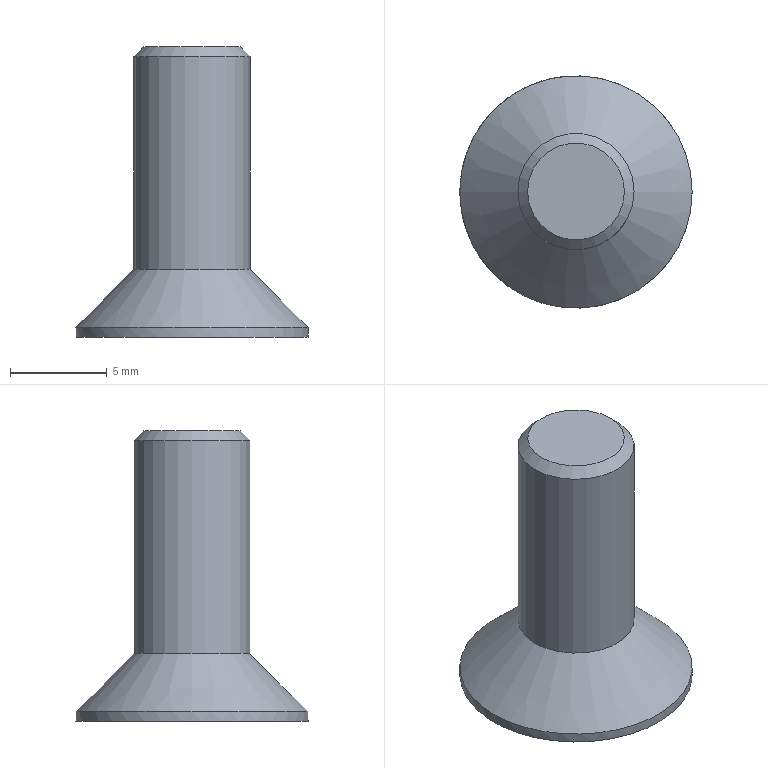Part | STEP file | LJD_id162_x_t | 1 solid | 13 faces | box 12 x 12 x 15 mm | volume 521.973 mm3 | plane 9 | cylinder 2 | cone 2 | commonest cylinder face diameters 6 x1 12 x1
STEP:
#1=CARTESIAN_POINT('',(61.,0.,-165.25));
#2=VERTEX_POINT('',#1);
#3=CARTESIAN_POINT('',(55.,0.,-165.25));
#4=DIRECTION('',(0.,0.,1.));
#5=DIRECTION('',(1.,0.,0.));
#6=AXIS2_PLACEMENT_3D('',#3,#4,#5);
#7=CIRCLE('',#6,6.);
#8=EDGE_CURVE('',#2,#2,#7,.T.);
#9=ORIENTED_EDGE('',*,*,#8,.F.);
#10=EDGE_LOOP('',(#9));
#11=FACE_BOUND('',#10,.T.);
#12=CARTESIAN_POINT('',(53.,-1.155,-165.25));
#13=VERTEX_POINT('',#12);
#14=CARTESIAN_POINT('',(55.,-2.309,-165.25));
#15=VERTEX_POINT('',#14);
#16=CARTESIAN_POINT('',(53.,-1.155,-165.25));
#17=DIRECTION('',(0.866,-0.5,0.));
#18=VECTOR('',#17,1.);
#19=LINE('',#16,#18);
#20=EDGE_CURVE('',#13,#15,#19,.T.);
#21=ORIENTED_EDGE('',*,*,#20,.T.);
#22=CARTESIAN_POINT('',(57.,-1.155,-165.25));
#23=VERTEX_POINT('',#22);
#24=CARTESIAN_POINT('',(55.,-2.309,-165.25));
#25=DIRECTION('',(0.866,0.5,0.));
#26=VECTOR('',#25,1.);
#27=LINE('',#24,#26);
#28=EDGE_CURVE('',#15,#23,#27,.T.);
#29=ORIENTED_EDGE('',*,*,#28,.T.);
#30=CARTESIAN_POINT('',(57.,1.155,-165.25));
#31=VERTEX_POINT('',#30);
#32=CARTESIAN_POINT('',(57.,-1.155,-165.25));
#33=DIRECTION('',(0.,1.,0.));
#34=VECTOR('',#33,1.);
#35=LINE('',#32,#34);
#36=EDGE_CURVE('',#23,#31,#35,.T.);
#37=ORIENTED_EDGE('',*,*,#36,.T.);
#38=CARTESIAN_POINT('',(55.,2.309,-165.25));
#39=VERTEX_POINT('',#38);
#40=CARTESIAN_POINT('',(57.,1.155,-165.25));
#41=DIRECTION('',(-0.866,0.5,0.));
#42=VECTOR('',#41,1.);
#43=LINE('',#40,#42);
#44=EDGE_CURVE('',#31,#39,#43,.T.);
#45=ORIENTED_EDGE('',*,*,#44,.T.);
#46=CARTESIAN_POINT('',(53.,1.155,-165.25));
#47=VERTEX_POINT('',#46);
#48=CARTESIAN_POINT('',(55.,2.309,-165.25));
#49=DIRECTION('',(-0.866,-0.5,0.));
#50=VECTOR('',#49,1.);
#51=LINE('',#48,#50);
#52=EDGE_CURVE('',#39,#47,#51,.T.);
#53=ORIENTED_EDGE('',*,*,#52,.T.);
#54=CARTESIAN_POINT('',(53.,1.155,-165.25));
#55=DIRECTION('',(0.,-1.,0.));
#56=VECTOR('',#55,1.);
#57=LINE('',#54,#56);
#58=EDGE_CURVE('',#47,#13,#57,.T.);
#59=ORIENTED_EDGE('',*,*,#58,.T.);
#60=EDGE_LOOP('',(#21,#29,#37,#45,#53,#59));
#61=FACE_BOUND('',#60,.T.);
#62=CARTESIAN_POINT('',(55.,0.,-165.25));
#63=DIRECTION('',(0.,0.,-1.));
#64=DIRECTION('',(-1.,0.,0.));
#65=AXIS2_PLACEMENT_3D('',#62,#63,#64);
#66=PLANE('',#65);
#67=ADVANCED_FACE('',(#11,#61),#66,.T.);
#68=CARTESIAN_POINT('',(61.,0.,-164.75));
#69=VERTEX_POINT('',#68);
#70=CARTESIAN_POINT('',(55.,0.,-164.75));
#71=DIRECTION('',(0.,0.,1.));
#72=DIRECTION('',(1.,0.,0.));
#73=AXIS2_PLACEMENT_3D('',#70,#71,#72);
#74=CIRCLE('',#73,6.);
#75=EDGE_CURVE('',#69,#69,#74,.T.);
#76=ORIENTED_EDGE('',*,*,#75,.F.);
#77=EDGE_LOOP('',(#76));
#78=FACE_BOUND('',#77,.T.);
#79=ORIENTED_EDGE('',*,*,#8,.T.);
#80=EDGE_LOOP('',(#79));
#81=FACE_BOUND('',#80,.T.);
#82=CARTESIAN_POINT('',(55.,0.,-165.25));
#83=DIRECTION('',(0.,0.,1.));
#84=DIRECTION('',(1.,0.,0.));
#85=AXIS2_PLACEMENT_3D('',#82,#83,#84);
#86=CYLINDRICAL_SURFACE('',#85,6.);
#87=ADVANCED_FACE('',(#78,#81),#86,.T.);
#88=ORIENTED_EDGE('',*,*,#75,.T.);
#89=EDGE_LOOP('',(#88));
#90=FACE_BOUND('',#89,.T.);
#91=CARTESIAN_POINT('',(52.,0.,-161.75));
#92=VERTEX_POINT('',#91);
#93=CARTESIAN_POINT('',(55.,0.,-161.75));
#94=DIRECTION('',(0.,0.,1.));
#95=DIRECTION('',(-1.,0.,0.));
#96=AXIS2_PLACEMENT_3D('',#93,#94,#95);
#97=CIRCLE('',#96,3.);
#98=EDGE_CURVE('',#92,#92,#97,.T.);
#99=ORIENTED_EDGE('',*,*,#98,.F.);
#100=EDGE_LOOP('',(#99));
#101=FACE_BOUND('',#100,.T.);
#102=CARTESIAN_POINT('',(55.,0.,-161.75));
#103=DIRECTION('',(0.,0.,-1.));
#104=DIRECTION('',(-1.,0.,0.));
#105=AXIS2_PLACEMENT_3D('',#102,#103,#104);
#106=CONICAL_SURFACE('',#105,3.,45.);
#107=ADVANCED_FACE('',(#90,#101),#106,.T.);
#108=CARTESIAN_POINT('',(57.5,0.,-150.25));
#109=VERTEX_POINT('',#108);
#110=CARTESIAN_POINT('',(55.,0.,-150.25));
#111=DIRECTION('',(0.,0.,1.));
#112=DIRECTION('',(1.,0.,0.));
#113=AXIS2_PLACEMENT_3D('',#110,#111,#112);
#114=CIRCLE('',#113,2.5);
#115=EDGE_CURVE('',#109,#109,#114,.T.);
#116=ORIENTED_EDGE('',*,*,#115,.T.);
#117=EDGE_LOOP('',(#116));
#118=FACE_OUTER_BOUND('',#117,.T.);
#119=CARTESIAN_POINT('',(55.,0.,-150.25));
#120=DIRECTION('',(0.,0.,1.));
#121=DIRECTION('',(1.,0.,0.));
#122=AXIS2_PLACEMENT_3D('',#119,#120,#121);
#123=PLANE('',#122);
#124=ADVANCED_FACE('',(#118),#123,.T.);
#125=CARTESIAN_POINT('',(58.,0.,-150.75));
#126=VERTEX_POINT('',#125);
#127=CARTESIAN_POINT('',(55.,0.,-150.75));
#128=DIRECTION('',(0.,0.,-1.));
#129=DIRECTION('',(1.,0.,0.));
#130=AXIS2_PLACEMENT_3D('',#127,#128,#129);
#131=CIRCLE('',#130,3.);
#132=EDGE_CURVE('',#126,#126,#131,.T.);
#133=ORIENTED_EDGE('',*,*,#132,.T.);
#134=EDGE_LOOP('',(#133));
#135=FACE_BOUND('',#134,.T.);
#136=ORIENTED_EDGE('',*,*,#98,.T.);
#137=EDGE_LOOP('',(#136));
#138=FACE_BOUND('',#137,.T.);
#139=CARTESIAN_POINT('',(55.,0.,-165.25));
#140=DIRECTION('',(0.,0.,1.));
#141=DIRECTION('',(1.,0.,0.));
#142=AXIS2_PLACEMENT_3D('',#139,#140,#141);
#143=CYLINDRICAL_SURFACE('',#142,3.);
#144=ADVANCED_FACE('',(#135,#138),#143,.T.);
#145=CARTESIAN_POINT('',(53.,-1.155,-161.25));
#146=VERTEX_POINT('',#145);
#147=CARTESIAN_POINT('',(55.,-2.309,-161.25));
#148=VERTEX_POINT('',#147);
#149=CARTESIAN_POINT('',(53.,-1.155,-161.25));
#150=DIRECTION('',(0.866,-0.5,0.));
#151=VECTOR('',#150,1.);
#152=LINE('',#149,#151);
#153=EDGE_CURVE('',#146,#148,#152,.T.);
#154=ORIENTED_EDGE('',*,*,#153,.T.);
#155=CARTESIAN_POINT('',(55.,-2.309,-165.25));
#156=DIRECTION('',(0.,0.,1.));
#157=VECTOR('',#156,1.);
#158=LINE('',#155,#157);
#159=EDGE_CURVE('',#15,#148,#158,.T.);
#160=ORIENTED_EDGE('',*,*,#159,.F.);
#161=ORIENTED_EDGE('',*,*,#20,.F.);
#162=CARTESIAN_POINT('',(53.,-1.155,-165.25));
#163=DIRECTION('',(0.,0.,1.));
#164=VECTOR('',#163,1.);
#165=LINE('',#162,#164);
#166=EDGE_CURVE('',#13,#146,#165,.T.);
#167=ORIENTED_EDGE('',*,*,#166,.T.);
#168=EDGE_LOOP('',(#154,#160,#161,#167));
#169=FACE_OUTER_BOUND('',#168,.T.);
#170=CARTESIAN_POINT('',(54.,-1.732,-163.25));
#171=DIRECTION('',(-0.5,-0.866,0.));
#172=DIRECTION('',(0.866,-0.5,0.));
#173=AXIS2_PLACEMENT_3D('',#170,#171,#172);
#174=PLANE('',#173);
#175=ADVANCED_FACE('',(#169),#174,.F.);
#176=CARTESIAN_POINT('',(53.,1.155,-161.25));
#177=VERTEX_POINT('',#176);
#178=CARTESIAN_POINT('',(53.,1.155,-161.25));
#179=DIRECTION('',(0.,-1.,0.));
#180=VECTOR('',#179,1.);
#181=LINE('',#178,#180);
#182=EDGE_CURVE('',#177,#146,#181,.T.);
#183=ORIENTED_EDGE('',*,*,#182,.T.);
#184=ORIENTED_EDGE('',*,*,#166,.F.);
#185=ORIENTED_EDGE('',*,*,#58,.F.);
#186=CARTESIAN_POINT('',(53.,1.155,-165.25));
#187=DIRECTION('',(0.,0.,1.));
#188=VECTOR('',#187,1.);
#189=LINE('',#186,#188);
#190=EDGE_CURVE('',#47,#177,#189,.T.);
#191=ORIENTED_EDGE('',*,*,#190,.T.);
#192=EDGE_LOOP('',(#183,#184,#185,#191));
#193=FACE_OUTER_BOUND('',#192,.T.);
#194=CARTESIAN_POINT('',(53.,0.,-163.25));
#195=DIRECTION('',(-1.,0.,0.));
#196=DIRECTION('',(0.,0.,1.));
#197=AXIS2_PLACEMENT_3D('',#194,#195,#196);
#198=PLANE('',#197);
#199=ADVANCED_FACE('',(#193),#198,.F.);
#200=CARTESIAN_POINT('',(55.,2.309,-161.25));
#201=VERTEX_POINT('',#200);
#202=CARTESIAN_POINT('',(55.,2.309,-161.25));
#203=DIRECTION('',(-0.866,-0.5,0.));
#204=VECTOR('',#203,1.);
#205=LINE('',#202,#204);
#206=EDGE_CURVE('',#201,#177,#205,.T.);
#207=ORIENTED_EDGE('',*,*,#206,.T.);
#208=ORIENTED_EDGE('',*,*,#190,.F.);
#209=ORIENTED_EDGE('',*,*,#52,.F.);
#210=CARTESIAN_POINT('',(55.,2.309,-165.25));
#211=DIRECTION('',(0.,0.,1.));
#212=VECTOR('',#211,1.);
#213=LINE('',#210,#212);
#214=EDGE_CURVE('',#39,#201,#213,.T.);
#215=ORIENTED_EDGE('',*,*,#214,.T.);
#216=EDGE_LOOP('',(#207,#208,#209,#215));
#217=FACE_OUTER_BOUND('',#216,.T.);
#218=CARTESIAN_POINT('',(54.,1.732,-163.25));
#219=DIRECTION('',(-0.5,0.866,0.));
#220=DIRECTION('',(-0.866,-0.5,0.));
#221=AXIS2_PLACEMENT_3D('',#218,#219,#220);
#222=PLANE('',#221);
#223=ADVANCED_FACE('',(#217),#222,.F.);
#224=CARTESIAN_POINT('',(57.,1.155,-161.25));
#225=VERTEX_POINT('',#224);
#226=CARTESIAN_POINT('',(57.,1.155,-161.25));
#227=DIRECTION('',(-0.866,0.5,0.));
#228=VECTOR('',#227,1.);
#229=LINE('',#226,#228);
#230=EDGE_CURVE('',#225,#201,#229,.T.);
#231=ORIENTED_EDGE('',*,*,#230,.T.);
#232=ORIENTED_EDGE('',*,*,#214,.F.);
#233=ORIENTED_EDGE('',*,*,#44,.F.);
#234=CARTESIAN_POINT('',(57.,1.155,-165.25));
#235=DIRECTION('',(0.,0.,1.));
#236=VECTOR('',#235,1.);
#237=LINE('',#234,#236);
#238=EDGE_CURVE('',#31,#225,#237,.T.);
#239=ORIENTED_EDGE('',*,*,#238,.T.);
#240=EDGE_LOOP('',(#231,#232,#233,#239));
#241=FACE_OUTER_BOUND('',#240,.T.);
#242=CARTESIAN_POINT('',(56.,1.732,-163.25));
#243=DIRECTION('',(0.5,0.866,0.));
#244=DIRECTION('',(-0.866,0.5,0.));
#245=AXIS2_PLACEMENT_3D('',#242,#243,#244);
#246=PLANE('',#245);
#247=ADVANCED_FACE('',(#241),#246,.F.);
#248=CARTESIAN_POINT('',(57.,-1.155,-161.25));
#249=VERTEX_POINT('',#248);
#250=CARTESIAN_POINT('',(57.,-1.155,-161.25));
#251=DIRECTION('',(0.,1.,0.));
#252=VECTOR('',#251,1.);
#253=LINE('',#250,#252);
#254=EDGE_CURVE('',#249,#225,#253,.T.);
#255=ORIENTED_EDGE('',*,*,#254,.T.);
#256=ORIENTED_EDGE('',*,*,#238,.F.);
#257=ORIENTED_EDGE('',*,*,#36,.F.);
#258=CARTESIAN_POINT('',(57.,-1.155,-165.25));
#259=DIRECTION('',(0.,0.,1.));
#260=VECTOR('',#259,1.);
#261=LINE('',#258,#260);
#262=EDGE_CURVE('',#23,#249,#261,.T.);
#263=ORIENTED_EDGE('',*,*,#262,.T.);
#264=EDGE_LOOP('',(#255,#256,#257,#263));
#265=FACE_OUTER_BOUND('',#264,.T.);
#266=CARTESIAN_POINT('',(57.,0.,-163.25));
#267=DIRECTION('',(1.,0.,0.));
#268=DIRECTION('',(0.,0.,-1.));
#269=AXIS2_PLACEMENT_3D('',#266,#267,#268);
#270=PLANE('',#269);
#271=ADVANCED_FACE('',(#265),#270,.F.);
#272=CARTESIAN_POINT('',(55.,-2.309,-161.25));
#273=DIRECTION('',(0.866,0.5,0.));
#274=VECTOR('',#273,1.);
#275=LINE('',#272,#274);
#276=EDGE_CURVE('',#148,#249,#275,.T.);
#277=ORIENTED_EDGE('',*,*,#276,.T.);
#278=ORIENTED_EDGE('',*,*,#262,.F.);
#279=ORIENTED_EDGE('',*,*,#28,.F.);
#280=ORIENTED_EDGE('',*,*,#159,.T.);
#281=EDGE_LOOP('',(#277,#278,#279,#280));
#282=FACE_OUTER_BOUND('',#281,.T.);
#283=CARTESIAN_POINT('',(56.,-1.732,-163.25));
#284=DIRECTION('',(0.5,-0.866,0.));
#285=DIRECTION('',(0.866,0.5,0.));
#286=AXIS2_PLACEMENT_3D('',#283,#284,#285);
#287=PLANE('',#286);
#288=ADVANCED_FACE('',(#282),#287,.F.);
#289=ORIENTED_EDGE('',*,*,#182,.F.);
#290=ORIENTED_EDGE('',*,*,#206,.F.);
#291=ORIENTED_EDGE('',*,*,#230,.F.);
#292=ORIENTED_EDGE('',*,*,#254,.F.);
#293=ORIENTED_EDGE('',*,*,#276,.F.);
#294=ORIENTED_EDGE('',*,*,#153,.F.);
#295=EDGE_LOOP('',(#289,#290,#291,#292,#293,#294));
#296=FACE_OUTER_BOUND('',#295,.T.);
#297=CARTESIAN_POINT('',(55.,0.,-161.25));
#298=DIRECTION('',(0.,0.,1.));
#299=DIRECTION('',(1.,0.,0.));
#300=AXIS2_PLACEMENT_3D('',#297,#298,#299);
#301=PLANE('',#300);
#302=ADVANCED_FACE('',(#296),#301,.F.);
#303=ORIENTED_EDGE('',*,*,#115,.F.);
#304=EDGE_LOOP('',(#303));
#305=FACE_BOUND('',#304,.T.);
#306=ORIENTED_EDGE('',*,*,#132,.F.);
#307=EDGE_LOOP('',(#306));
#308=FACE_BOUND('',#307,.T.);
#309=CARTESIAN_POINT('',(55.,0.,-150.75));
#310=DIRECTION('',(0.,0.,-1.));
#311=DIRECTION('',(-1.,0.,0.));
#312=AXIS2_PLACEMENT_3D('',#309,#310,#311);
#313=CONICAL_SURFACE('',#312,3.,45.);
#314=ADVANCED_FACE('',(#305,#308),#313,.T.);
#315=CLOSED_SHELL('',(#67,#87,#107,#124,#144,#175,#199,#223,#247,#271,#288,#302,#314));
#316=MANIFOLD_SOLID_BREP('',#315);
#317=(LENGTH_UNIT()NAMED_UNIT(*)SI_UNIT(.MILLI.,.METRE.));
#318=UNCERTAINTY_MEASURE_WITH_UNIT(LENGTH_MEASURE(0.00002),#317,'','');
#319=(NAMED_UNIT(*)PLANE_ANGLE_UNIT()SI_UNIT($,.RADIAN.));
#320=PLANE_ANGLE_MEASURE_WITH_UNIT(PLANE_ANGLE_MEASURE(0.01745),#319);
#321=DIMENSIONAL_EXPONENTS(0.,0.,0.,0.,0.,0.,0.);
#322=(CONVERSION_BASED_UNIT('DEGREE',#320)NAMED_UNIT(#321)PLANE_ANGLE_UNIT());
#323=(NAMED_UNIT(*)SI_UNIT($,.STERADIAN.)SOLID_ANGLE_UNIT());
#324=(GEOMETRIC_REPRESENTATION_CONTEXT(3)GLOBAL_UNCERTAINTY_ASSIGNED_CONTEXT((#318))GLOBAL_UNIT_ASSIGNED_CONTEXT((#317,#322,#323))REPRESENTATION_CONTEXT('',''));
#325=ADVANCED_BREP_SHAPE_REPRESENTATION('',(#316),#324);